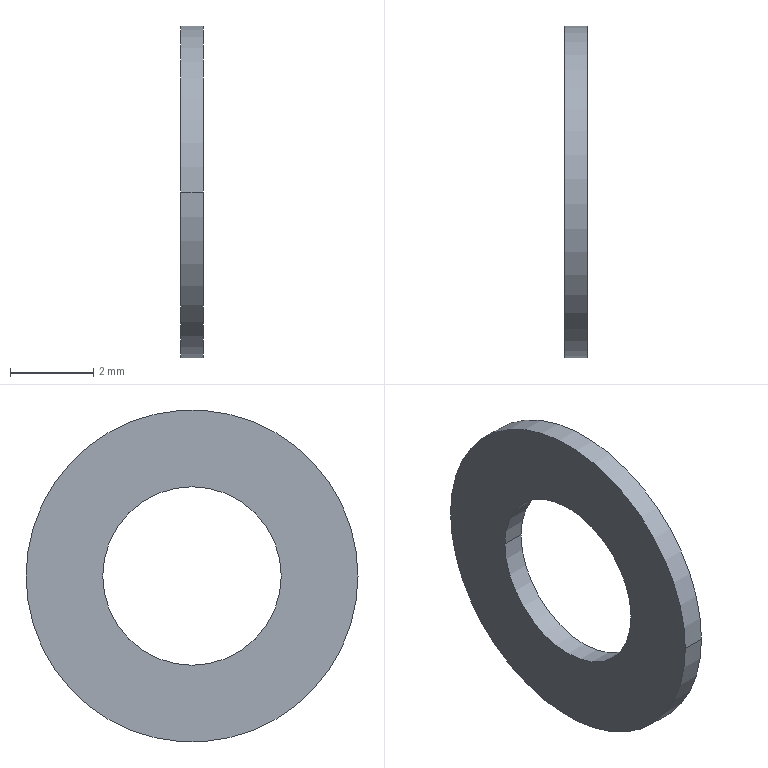Part | STEP file | DINENISO7092-4 | 1 solid | 6 faces | box 0.55 x 8 x 8 mm | volume 19.659 mm3 | cylinder 4 | plane 2 | commonest cylinder face diameters 4.3 x2 8 x2
STEP:
#1=CARTESIAN_POINT('',(0.,0.,0.));
#2=DIRECTION('',(0.,0.,1.));
#3=DIRECTION('',(1.,0.,0.));
#4=AXIS2_PLACEMENT_3D('',#1,#2,#3);
#5=CARTESIAN_POINT('',(0.,0.,0.));
#6=VERTEX_POINT('',#5);
#7=CARTESIAN_POINT('',(0.,-8.,0.));
#8=VERTEX_POINT('',#7);
#9=CARTESIAN_POINT('',(0.,-4.,0.));
#10=DIRECTION('',(-1.,0.,0.));
#11=DIRECTION('',(0.,1.,0.));
#12=AXIS2_PLACEMENT_3D('',#9,#10,#11);
#13=CIRCLE('',#12,4.);
#14=CARTESIAN_POINT('',(0.,-4.,0.));
#15=DIRECTION('',(-1.,0.,0.));
#16=DIRECTION('',(0.,1.,0.));
#17=AXIS2_PLACEMENT_3D('',#14,#15,#16);
#18=PLANE('',#17);
#19=CARTESIAN_POINT('',(0.,0.));
#20=DIRECTION('',(1.,0.));
#21=AXIS2_PLACEMENT_2D('',#19,#20);
#22=CIRCLE('',#21,4.);
#23=(GEOMETRIC_REPRESENTATION_CONTEXT(2)PARAMETRIC_REPRESENTATION_CONTEXT()REPRESENTATION_CONTEXT('',''));
#24=DEFINITIONAL_REPRESENTATION('',(#22),#23);
#25=PCURVE('',#18,#24);
#26=CARTESIAN_POINT('',(0.5775,-4.,0.));
#27=DIRECTION('',(-1.,0.,0.));
#28=DIRECTION('',(0.,1.,0.));
#29=AXIS2_PLACEMENT_3D('',#26,#27,#28);
#30=CYLINDRICAL_SURFACE('',#29,4.);
#31=CARTESIAN_POINT('',(0.,0.5775));
#32=DIRECTION('',(1.,0.));
#33=VECTOR('',#32,1.);
#34=LINE('',#31,#33);
#35=(GEOMETRIC_REPRESENTATION_CONTEXT(2)PARAMETRIC_REPRESENTATION_CONTEXT()REPRESENTATION_CONTEXT('',''));
#36=DEFINITIONAL_REPRESENTATION('',(#34),#35);
#37=PCURVE('',#30,#36);
#38=SURFACE_CURVE('',#13,(#25,#37),.PCURVE_S1.);
#39=EDGE_CURVE('',#6,#8,#38,.T.);
#40=ORIENTED_EDGE('',*,*,#39,.F.);
#41=CARTESIAN_POINT('',(0.,-4.,0.));
#42=DIRECTION('',(1.,0.,0.));
#43=DIRECTION('',(0.,1.,0.));
#44=AXIS2_PLACEMENT_3D('',#41,#42,#43);
#45=CIRCLE('',#44,4.);
#46=CARTESIAN_POINT('',(4.,0.));
#47=CARTESIAN_POINT('',(4.,-6.928));
#48=CARTESIAN_POINT('',(-2.,-3.464));
#49=CARTESIAN_POINT('',(-8.,0.));
#50=CARTESIAN_POINT('',(-2.,3.464));
#51=CARTESIAN_POINT('',(4.,6.928));
#52=CARTESIAN_POINT('',(4.,0.));
#53=(BOUNDED_CURVE()B_SPLINE_CURVE(2,(#46,#47,#48,#49,#50,#51,#52),.UNSPECIFIED.,.T.,.F.)B_SPLINE_CURVE_WITH_KNOTS((1,2,2,2,2,1),(-2.094,0.,2.094,4.189,6.283,8.378),.UNSPECIFIED.)CURVE()GEOMETRIC_REPRESENTATION_ITEM()RATIONAL_B_SPLINE_CURVE((1.,0.5,1.,0.5,1.,0.5,1.))REPRESENTATION_ITEM(''));
#54=(GEOMETRIC_REPRESENTATION_CONTEXT(2)PARAMETRIC_REPRESENTATION_CONTEXT()REPRESENTATION_CONTEXT('',''));
#55=DEFINITIONAL_REPRESENTATION('',(#53),#54);
#56=PCURVE('',#18,#55);
#57=CARTESIAN_POINT('',(0.5775,-4.,0.));
#58=DIRECTION('',(-1.,0.,0.));
#59=DIRECTION('',(0.,1.,0.));
#60=AXIS2_PLACEMENT_3D('',#57,#58,#59);
#61=CYLINDRICAL_SURFACE('',#60,4.);
#62=CARTESIAN_POINT('',(6.283,0.5775));
#63=DIRECTION('',(-1.,0.));
#64=VECTOR('',#63,1.);
#65=LINE('',#62,#64);
#66=(GEOMETRIC_REPRESENTATION_CONTEXT(2)PARAMETRIC_REPRESENTATION_CONTEXT()REPRESENTATION_CONTEXT('',''));
#67=DEFINITIONAL_REPRESENTATION('',(#65),#66);
#68=PCURVE('',#61,#67);
#69=SURFACE_CURVE('',#45,(#56,#68),.PCURVE_S1.);
#70=EDGE_CURVE('',#6,#8,#69,.T.);
#71=ORIENTED_EDGE('',*,*,#70,.T.);
#72=EDGE_LOOP('',(#40,#71));
#73=FACE_BOUND('',#72,.F.);
#74=CARTESIAN_POINT('',(0.,-1.85,0.));
#75=VERTEX_POINT('',#74);
#76=CARTESIAN_POINT('',(0.,-6.15,0.));
#77=VERTEX_POINT('',#76);
#78=CARTESIAN_POINT('',(0.,-4.,0.));
#79=DIRECTION('',(1.,0.,0.));
#80=DIRECTION('',(0.,1.,0.));
#81=AXIS2_PLACEMENT_3D('',#78,#79,#80);
#82=CIRCLE('',#81,2.15);
#83=CARTESIAN_POINT('',(2.15,0.));
#84=CARTESIAN_POINT('',(2.15,-3.724));
#85=CARTESIAN_POINT('',(-1.075,-1.862));
#86=CARTESIAN_POINT('',(-4.3,0.));
#87=CARTESIAN_POINT('',(-1.075,1.862));
#88=CARTESIAN_POINT('',(2.15,3.724));
#89=CARTESIAN_POINT('',(2.15,0.));
#90=(BOUNDED_CURVE()B_SPLINE_CURVE(2,(#83,#84,#85,#86,#87,#88,#89),.UNSPECIFIED.,.T.,.F.)B_SPLINE_CURVE_WITH_KNOTS((1,2,2,2,2,1),(-2.094,0.,2.094,4.189,6.283,8.378),.UNSPECIFIED.)CURVE()GEOMETRIC_REPRESENTATION_ITEM()RATIONAL_B_SPLINE_CURVE((1.,0.5,1.,0.5,1.,0.5,1.))REPRESENTATION_ITEM(''));
#91=(GEOMETRIC_REPRESENTATION_CONTEXT(2)PARAMETRIC_REPRESENTATION_CONTEXT()REPRESENTATION_CONTEXT('',''));
#92=DEFINITIONAL_REPRESENTATION('',(#90),#91);
#93=PCURVE('',#18,#92);
#94=CARTESIAN_POINT('',(0.5775,-4.,0.));
#95=DIRECTION('',(-1.,0.,0.));
#96=DIRECTION('',(0.,1.,0.));
#97=AXIS2_PLACEMENT_3D('',#94,#95,#96);
#98=CYLINDRICAL_SURFACE('',#97,2.15);
#99=CARTESIAN_POINT('',(6.283,0.5775));
#100=DIRECTION('',(-1.,0.));
#101=VECTOR('',#100,1.);
#102=LINE('',#99,#101);
#103=(GEOMETRIC_REPRESENTATION_CONTEXT(2)PARAMETRIC_REPRESENTATION_CONTEXT()REPRESENTATION_CONTEXT('',''));
#104=DEFINITIONAL_REPRESENTATION('',(#102),#103);
#105=PCURVE('',#98,#104);
#106=SURFACE_CURVE('',#82,(#93,#105),.PCURVE_S1.);
#107=EDGE_CURVE('',#75,#77,#106,.T.);
#108=ORIENTED_EDGE('',*,*,#107,.F.);
#109=CARTESIAN_POINT('',(0.,-4.,0.));
#110=DIRECTION('',(-1.,0.,0.));
#111=DIRECTION('',(0.,1.,0.));
#112=AXIS2_PLACEMENT_3D('',#109,#110,#111);
#113=CIRCLE('',#112,2.15);
#114=CARTESIAN_POINT('',(0.,0.));
#115=DIRECTION('',(1.,0.));
#116=AXIS2_PLACEMENT_2D('',#114,#115);
#117=CIRCLE('',#116,2.15);
#118=(GEOMETRIC_REPRESENTATION_CONTEXT(2)PARAMETRIC_REPRESENTATION_CONTEXT()REPRESENTATION_CONTEXT('',''));
#119=DEFINITIONAL_REPRESENTATION('',(#117),#118);
#120=PCURVE('',#18,#119);
#121=CARTESIAN_POINT('',(0.5775,-4.,0.));
#122=DIRECTION('',(-1.,0.,0.));
#123=DIRECTION('',(0.,1.,0.));
#124=AXIS2_PLACEMENT_3D('',#121,#122,#123);
#125=CYLINDRICAL_SURFACE('',#124,2.15);
#126=CARTESIAN_POINT('',(0.,0.5775));
#127=DIRECTION('',(1.,0.));
#128=VECTOR('',#127,1.);
#129=LINE('',#126,#128);
#130=(GEOMETRIC_REPRESENTATION_CONTEXT(2)PARAMETRIC_REPRESENTATION_CONTEXT()REPRESENTATION_CONTEXT('',''));
#131=DEFINITIONAL_REPRESENTATION('',(#129),#130);
#132=PCURVE('',#125,#131);
#133=SURFACE_CURVE('',#113,(#120,#132),.PCURVE_S1.);
#134=EDGE_CURVE('',#75,#77,#133,.T.);
#135=ORIENTED_EDGE('',*,*,#134,.T.);
#136=EDGE_LOOP('',(#108,#135));
#137=FACE_BOUND('',#136,.F.);
#138=ADVANCED_FACE('',(#73,#137),#18,.T.);
#139=CARTESIAN_POINT('',(0.55,0.,0.));
#140=VERTEX_POINT('',#139);
#141=CARTESIAN_POINT('',(0.55,-8.,0.));
#142=VERTEX_POINT('',#141);
#143=CARTESIAN_POINT('',(0.55,-4.,0.));
#144=DIRECTION('',(-1.,0.,0.));
#145=DIRECTION('',(0.,1.,0.));
#146=AXIS2_PLACEMENT_3D('',#143,#144,#145);
#147=CIRCLE('',#146,4.);
#148=CARTESIAN_POINT('',(0.,0.0275));
#149=DIRECTION('',(1.,0.));
#150=VECTOR('',#149,1.);
#151=LINE('',#148,#150);
#152=(GEOMETRIC_REPRESENTATION_CONTEXT(2)PARAMETRIC_REPRESENTATION_CONTEXT()REPRESENTATION_CONTEXT('',''));
#153=DEFINITIONAL_REPRESENTATION('',(#151),#152);
#154=PCURVE('',#30,#153);
#155=CARTESIAN_POINT('',(0.55,-4.,0.));
#156=DIRECTION('',(-1.,0.,0.));
#157=DIRECTION('',(0.,1.,0.));
#158=AXIS2_PLACEMENT_3D('',#155,#156,#157);
#159=PLANE('',#158);
#160=CARTESIAN_POINT('',(0.,0.));
#161=DIRECTION('',(1.,0.));
#162=AXIS2_PLACEMENT_2D('',#160,#161);
#163=CIRCLE('',#162,4.);
#164=(GEOMETRIC_REPRESENTATION_CONTEXT(2)PARAMETRIC_REPRESENTATION_CONTEXT()REPRESENTATION_CONTEXT('',''));
#165=DEFINITIONAL_REPRESENTATION('',(#163),#164);
#166=PCURVE('',#159,#165);
#167=SURFACE_CURVE('',#147,(#154,#166),.PCURVE_S1.);
#168=EDGE_CURVE('',#140,#142,#167,.T.);
#169=ORIENTED_EDGE('',*,*,#168,.T.);
#170=CARTESIAN_POINT('',(0.55,-8.,0.));
#171=DIRECTION('',(-1.,0.,0.));
#172=VECTOR('',#171,1.);
#173=LINE('',#170,#172);
#174=CARTESIAN_POINT('',(3.142,0.0275));
#175=DIRECTION('',(0.,1.));
#176=VECTOR('',#175,1.);
#177=LINE('',#174,#176);
#178=(GEOMETRIC_REPRESENTATION_CONTEXT(2)PARAMETRIC_REPRESENTATION_CONTEXT()REPRESENTATION_CONTEXT('',''));
#179=DEFINITIONAL_REPRESENTATION('',(#177),#178);
#180=PCURVE('',#30,#179);
#181=CARTESIAN_POINT('',(3.142,0.0275));
#182=DIRECTION('',(0.,1.));
#183=VECTOR('',#182,1.);
#184=LINE('',#181,#183);
#185=(GEOMETRIC_REPRESENTATION_CONTEXT(2)PARAMETRIC_REPRESENTATION_CONTEXT()REPRESENTATION_CONTEXT('',''));
#186=DEFINITIONAL_REPRESENTATION('',(#184),#185);
#187=PCURVE('',#61,#186);
#188=SURFACE_CURVE('',#173,(#180,#187),.PCURVE_S1.);
#189=EDGE_CURVE('',#142,#8,#188,.T.);
#190=ORIENTED_EDGE('',*,*,#189,.T.);
#191=ORIENTED_EDGE('',*,*,#39,.F.);
#192=CARTESIAN_POINT('',(0.55,0.,0.));
#193=DIRECTION('',(-1.,0.,0.));
#194=VECTOR('',#193,1.);
#195=LINE('',#192,#194);
#196=CARTESIAN_POINT('',(0.,0.0275));
#197=DIRECTION('',(0.,1.));
#198=VECTOR('',#197,1.);
#199=LINE('',#196,#198);
#200=(GEOMETRIC_REPRESENTATION_CONTEXT(2)PARAMETRIC_REPRESENTATION_CONTEXT()REPRESENTATION_CONTEXT('',''));
#201=DEFINITIONAL_REPRESENTATION('',(#199),#200);
#202=PCURVE('',#30,#201);
#203=CARTESIAN_POINT('',(6.283,0.0275));
#204=DIRECTION('',(0.,1.));
#205=VECTOR('',#204,1.);
#206=LINE('',#203,#205);
#207=(GEOMETRIC_REPRESENTATION_CONTEXT(2)PARAMETRIC_REPRESENTATION_CONTEXT()REPRESENTATION_CONTEXT('',''));
#208=DEFINITIONAL_REPRESENTATION('',(#206),#207);
#209=PCURVE('',#61,#208);
#210=SURFACE_CURVE('',#195,(#202,#209),.PCURVE_S1.);
#211=EDGE_CURVE('',#140,#6,#210,.T.);
#212=ORIENTED_EDGE('',*,*,#211,.F.);
#213=EDGE_LOOP('',(#169,#190,#191,#212));
#214=FACE_BOUND('',#213,.T.);
#215=ADVANCED_FACE('',(#214),#30,.T.);
#216=ORIENTED_EDGE('',*,*,#70,.T.);
#217=ORIENTED_EDGE('',*,*,#189,.F.);
#218=CARTESIAN_POINT('',(0.55,-4.,0.));
#219=DIRECTION('',(1.,0.,0.));
#220=DIRECTION('',(0.,1.,0.));
#221=AXIS2_PLACEMENT_3D('',#218,#219,#220);
#222=CIRCLE('',#221,4.);
#223=CARTESIAN_POINT('',(6.283,0.0275));
#224=DIRECTION('',(-1.,0.));
#225=VECTOR('',#224,1.);
#226=LINE('',#223,#225);
#227=(GEOMETRIC_REPRESENTATION_CONTEXT(2)PARAMETRIC_REPRESENTATION_CONTEXT()REPRESENTATION_CONTEXT('',''));
#228=DEFINITIONAL_REPRESENTATION('',(#226),#227);
#229=PCURVE('',#61,#228);
#230=CARTESIAN_POINT('',(4.,0.));
#231=CARTESIAN_POINT('',(4.,-6.928));
#232=CARTESIAN_POINT('',(-2.,-3.464));
#233=CARTESIAN_POINT('',(-8.,0.));
#234=CARTESIAN_POINT('',(-2.,3.464));
#235=CARTESIAN_POINT('',(4.,6.928));
#236=CARTESIAN_POINT('',(4.,0.));
#237=(BOUNDED_CURVE()B_SPLINE_CURVE(2,(#230,#231,#232,#233,#234,#235,#236),.UNSPECIFIED.,.T.,.F.)B_SPLINE_CURVE_WITH_KNOTS((1,2,2,2,2,1),(-2.094,0.,2.094,4.189,6.283,8.378),.UNSPECIFIED.)CURVE()GEOMETRIC_REPRESENTATION_ITEM()RATIONAL_B_SPLINE_CURVE((1.,0.5,1.,0.5,1.,0.5,1.))REPRESENTATION_ITEM(''));
#238=(GEOMETRIC_REPRESENTATION_CONTEXT(2)PARAMETRIC_REPRESENTATION_CONTEXT()REPRESENTATION_CONTEXT('',''));
#239=DEFINITIONAL_REPRESENTATION('',(#237),#238);
#240=PCURVE('',#159,#239);
#241=SURFACE_CURVE('',#222,(#229,#240),.PCURVE_S1.);
#242=EDGE_CURVE('',#140,#142,#241,.T.);
#243=ORIENTED_EDGE('',*,*,#242,.F.);
#244=ORIENTED_EDGE('',*,*,#211,.T.);
#245=EDGE_LOOP('',(#216,#217,#243,#244));
#246=FACE_BOUND('',#245,.T.);
#247=ADVANCED_FACE('',(#246),#61,.T.);
#248=ORIENTED_EDGE('',*,*,#242,.F.);
#249=ORIENTED_EDGE('',*,*,#168,.T.);
#250=EDGE_LOOP('',(#248,#249));
#251=FACE_BOUND('',#250,.F.);
#252=CARTESIAN_POINT('',(0.55,-1.85,0.));
#253=VERTEX_POINT('',#252);
#254=CARTESIAN_POINT('',(0.55,-6.15,0.));
#255=VERTEX_POINT('',#254);
#256=CARTESIAN_POINT('',(0.55,-4.,0.));
#257=DIRECTION('',(-1.,0.,0.));
#258=DIRECTION('',(0.,1.,0.));
#259=AXIS2_PLACEMENT_3D('',#256,#257,#258);
#260=CIRCLE('',#259,2.15);
#261=CARTESIAN_POINT('',(0.,0.));
#262=DIRECTION('',(1.,0.));
#263=AXIS2_PLACEMENT_2D('',#261,#262);
#264=CIRCLE('',#263,2.15);
#265=(GEOMETRIC_REPRESENTATION_CONTEXT(2)PARAMETRIC_REPRESENTATION_CONTEXT()REPRESENTATION_CONTEXT('',''));
#266=DEFINITIONAL_REPRESENTATION('',(#264),#265);
#267=PCURVE('',#159,#266);
#268=CARTESIAN_POINT('',(0.,0.0275));
#269=DIRECTION('',(1.,0.));
#270=VECTOR('',#269,1.);
#271=LINE('',#268,#270);
#272=(GEOMETRIC_REPRESENTATION_CONTEXT(2)PARAMETRIC_REPRESENTATION_CONTEXT()REPRESENTATION_CONTEXT('',''));
#273=DEFINITIONAL_REPRESENTATION('',(#271),#272);
#274=PCURVE('',#125,#273);
#275=SURFACE_CURVE('',#260,(#267,#274),.PCURVE_S1.);
#276=EDGE_CURVE('',#253,#255,#275,.T.);
#277=ORIENTED_EDGE('',*,*,#276,.F.);
#278=CARTESIAN_POINT('',(0.55,-4.,0.));
#279=DIRECTION('',(1.,0.,0.));
#280=DIRECTION('',(0.,1.,0.));
#281=AXIS2_PLACEMENT_3D('',#278,#279,#280);
#282=CIRCLE('',#281,2.15);
#283=CARTESIAN_POINT('',(2.15,0.));
#284=CARTESIAN_POINT('',(2.15,-3.724));
#285=CARTESIAN_POINT('',(-1.075,-1.862));
#286=CARTESIAN_POINT('',(-4.3,0.));
#287=CARTESIAN_POINT('',(-1.075,1.862));
#288=CARTESIAN_POINT('',(2.15,3.724));
#289=CARTESIAN_POINT('',(2.15,0.));
#290=(BOUNDED_CURVE()B_SPLINE_CURVE(2,(#283,#284,#285,#286,#287,#288,#289),.UNSPECIFIED.,.T.,.F.)B_SPLINE_CURVE_WITH_KNOTS((1,2,2,2,2,1),(-2.094,0.,2.094,4.189,6.283,8.378),.UNSPECIFIED.)CURVE()GEOMETRIC_REPRESENTATION_ITEM()RATIONAL_B_SPLINE_CURVE((1.,0.5,1.,0.5,1.,0.5,1.))REPRESENTATION_ITEM(''));
#291=(GEOMETRIC_REPRESENTATION_CONTEXT(2)PARAMETRIC_REPRESENTATION_CONTEXT()REPRESENTATION_CONTEXT('',''));
#292=DEFINITIONAL_REPRESENTATION('',(#290),#291);
#293=PCURVE('',#159,#292);
#294=CARTESIAN_POINT('',(6.283,0.0275));
#295=DIRECTION('',(-1.,0.));
#296=VECTOR('',#295,1.);
#297=LINE('',#294,#296);
#298=(GEOMETRIC_REPRESENTATION_CONTEXT(2)PARAMETRIC_REPRESENTATION_CONTEXT()REPRESENTATION_CONTEXT('',''));
#299=DEFINITIONAL_REPRESENTATION('',(#297),#298);
#300=PCURVE('',#98,#299);
#301=SURFACE_CURVE('',#282,(#293,#300),.PCURVE_S1.);
#302=EDGE_CURVE('',#253,#255,#301,.T.);
#303=ORIENTED_EDGE('',*,*,#302,.T.);
#304=EDGE_LOOP('',(#277,#303));
#305=FACE_BOUND('',#304,.F.);
#306=ADVANCED_FACE('',(#251,#305),#159,.F.);
#307=CARTESIAN_POINT('',(0.,-1.85,0.));
#308=DIRECTION('',(1.,0.,0.));
#309=VECTOR('',#308,1.);
#310=LINE('',#307,#309);
#311=CARTESIAN_POINT('',(0.,0.5775));
#312=DIRECTION('',(0.,-1.));
#313=VECTOR('',#312,1.);
#314=LINE('',#311,#313);
#315=(GEOMETRIC_REPRESENTATION_CONTEXT(2)PARAMETRIC_REPRESENTATION_CONTEXT()REPRESENTATION_CONTEXT('',''));
#316=DEFINITIONAL_REPRESENTATION('',(#314),#315);
#317=PCURVE('',#125,#316);
#318=CARTESIAN_POINT('',(6.283,0.5775));
#319=DIRECTION('',(0.,-1.));
#320=VECTOR('',#319,1.);
#321=LINE('',#318,#320);
#322=(GEOMETRIC_REPRESENTATION_CONTEXT(2)PARAMETRIC_REPRESENTATION_CONTEXT()REPRESENTATION_CONTEXT('',''));
#323=DEFINITIONAL_REPRESENTATION('',(#321),#322);
#324=PCURVE('',#98,#323);
#325=SURFACE_CURVE('',#310,(#317,#324),.PCURVE_S1.);
#326=EDGE_CURVE('',#75,#253,#325,.T.);
#327=ORIENTED_EDGE('',*,*,#326,.T.);
#328=ORIENTED_EDGE('',*,*,#276,.T.);
#329=CARTESIAN_POINT('',(0.,-6.15,0.));
#330=DIRECTION('',(1.,0.,0.));
#331=VECTOR('',#330,1.);
#332=LINE('',#329,#331);
#333=CARTESIAN_POINT('',(3.142,0.5775));
#334=DIRECTION('',(0.,-1.));
#335=VECTOR('',#334,1.);
#336=LINE('',#333,#335);
#337=(GEOMETRIC_REPRESENTATION_CONTEXT(2)PARAMETRIC_REPRESENTATION_CONTEXT()REPRESENTATION_CONTEXT('',''));
#338=DEFINITIONAL_REPRESENTATION('',(#336),#337);
#339=PCURVE('',#125,#338);
#340=CARTESIAN_POINT('',(3.142,0.5775));
#341=DIRECTION('',(0.,-1.));
#342=VECTOR('',#341,1.);
#343=LINE('',#340,#342);
#344=(GEOMETRIC_REPRESENTATION_CONTEXT(2)PARAMETRIC_REPRESENTATION_CONTEXT()REPRESENTATION_CONTEXT('',''));
#345=DEFINITIONAL_REPRESENTATION('',(#343),#344);
#346=PCURVE('',#98,#345);
#347=SURFACE_CURVE('',#332,(#339,#346),.PCURVE_S1.);
#348=EDGE_CURVE('',#77,#255,#347,.T.);
#349=ORIENTED_EDGE('',*,*,#348,.F.);
#350=ORIENTED_EDGE('',*,*,#134,.F.);
#351=EDGE_LOOP('',(#327,#328,#349,#350));
#352=FACE_BOUND('',#351,.F.);
#353=ADVANCED_FACE('',(#352),#125,.F.);
#354=ORIENTED_EDGE('',*,*,#326,.F.);
#355=ORIENTED_EDGE('',*,*,#107,.T.);
#356=ORIENTED_EDGE('',*,*,#348,.T.);
#357=ORIENTED_EDGE('',*,*,#302,.F.);
#358=EDGE_LOOP('',(#354,#355,#356,#357));
#359=FACE_BOUND('',#358,.F.);
#360=ADVANCED_FACE('',(#359),#98,.F.);
#361=CLOSED_SHELL('',(#138,#215,#247,#306,#353,#360));
#362=MANIFOLD_SOLID_BREP('',#361);
#363=(LENGTH_UNIT()NAMED_UNIT(*)SI_UNIT(.MILLI.,.METRE.));
#364=UNCERTAINTY_MEASURE_WITH_UNIT(LENGTH_MEASURE(0.0000001),#363,'','');
#365=(NAMED_UNIT(*)PLANE_ANGLE_UNIT()SI_UNIT($,.RADIAN.));
#366=(NAMED_UNIT(*)SI_UNIT($,.STERADIAN.)SOLID_ANGLE_UNIT());
#367=(GEOMETRIC_REPRESENTATION_CONTEXT(3)GLOBAL_UNCERTAINTY_ASSIGNED_CONTEXT((#364))GLOBAL_UNIT_ASSIGNED_CONTEXT((#363,#365,#366))REPRESENTATION_CONTEXT('',''));
#368=ADVANCED_BREP_SHAPE_REPRESENTATION('',(#4,#362),#367);